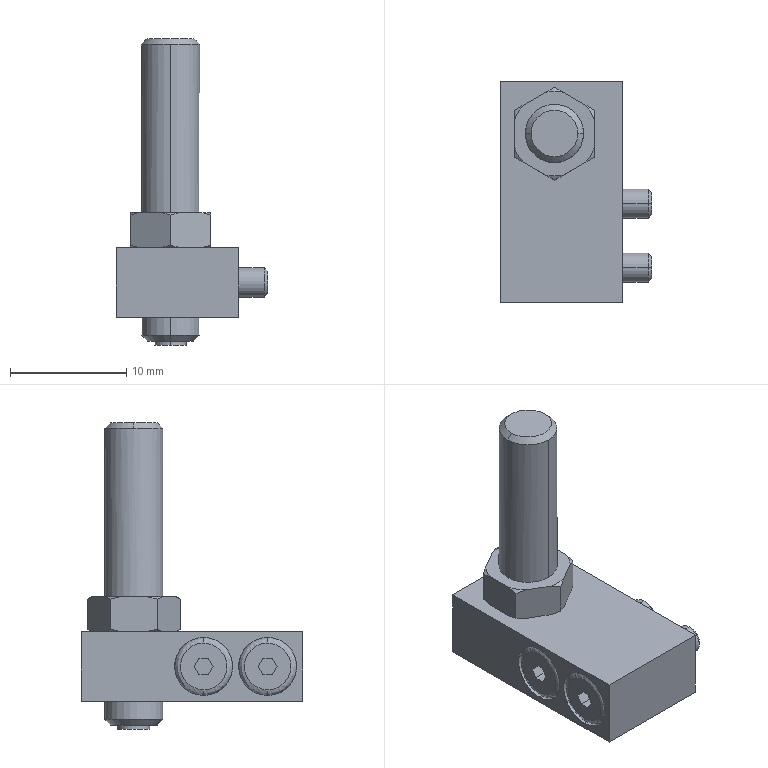Part | STEP file | QA-HI_MDX6_FB | 1 solid | 72 faces | box 13 x 19 x 26.37 mm | volume 1670 mm3 | plane 34 | cone 20 | cylinder 14 | spline 4 | commonest cylinder face diameters 5 x8 2.5 x4 2.744 x2